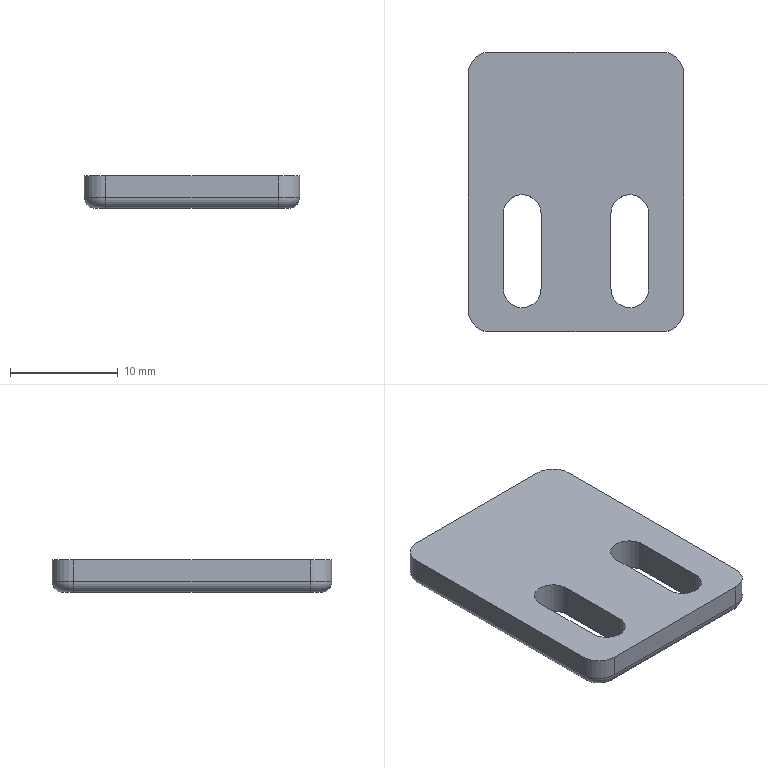Part | NX | 1 solid | 26 faces | box 20 x 26 x 3 mm | volume 1326 mm3 | cylinder 12 | plane 10 | torus 4 | commonest cylinder face diameters 2 x4 3.5 x4 4 x4
STEP:
#1=CARTESIAN_POINT('',(-3.25,-2.,1.5));
#2=VERTEX_POINT('',#1);
#3=CARTESIAN_POINT('',(-6.75,-2.,1.5));
#4=VERTEX_POINT('',#3);
#5=CARTESIAN_POINT('',(-5.,-2.,1.5));
#6=DIRECTION('',(0.,0.,1.));
#7=DIRECTION('',(1.,0.,0.));
#8=AXIS2_PLACEMENT_3D('',#5,#6,#7);
#9=CIRCLE('',#8,1.75);
#10=EDGE_CURVE('',#2,#4,#9,.T.);
#11=ORIENTED_EDGE('',*,*,#10,.F.);
#12=CARTESIAN_POINT('',(-3.25,-9.,1.5));
#13=VERTEX_POINT('',#12);
#14=CARTESIAN_POINT('',(-3.25,-2.,1.5));
#15=DIRECTION('',(0.,1.,0.));
#16=VECTOR('',#15,1000.);
#17=LINE('',#14,#16);
#18=EDGE_CURVE('',#13,#2,#17,.T.);
#19=ORIENTED_EDGE('',*,*,#18,.F.);
#20=CARTESIAN_POINT('',(-6.75,-9.,1.5));
#21=VERTEX_POINT('',#20);
#22=CARTESIAN_POINT('',(-5.,-9.,1.5));
#23=DIRECTION('',(0.,0.,1.));
#24=DIRECTION('',(1.,0.,0.));
#25=AXIS2_PLACEMENT_3D('',#22,#23,#24);
#26=CIRCLE('',#25,1.75);
#27=EDGE_CURVE('',#21,#13,#26,.T.);
#28=ORIENTED_EDGE('',*,*,#27,.F.);
#29=CARTESIAN_POINT('',(-6.75,-2.,1.5));
#30=DIRECTION('',(0.,-1.,0.));
#31=VECTOR('',#30,1000.);
#32=LINE('',#29,#31);
#33=EDGE_CURVE('',#4,#21,#32,.T.);
#34=ORIENTED_EDGE('',*,*,#33,.F.);
#35=EDGE_LOOP('',(#11,#19,#28,#34));
#36=FACE_BOUND('',#35,.T.);
#37=CARTESIAN_POINT('',(-10.,11.,1.5));
#38=VERTEX_POINT('',#37);
#39=CARTESIAN_POINT('',(-10.,-11.,1.5));
#40=VERTEX_POINT('',#39);
#41=CARTESIAN_POINT('',(-10.,13.,1.5));
#42=DIRECTION('',(0.,-1.,0.));
#43=VECTOR('',#42,1000.);
#44=LINE('',#41,#43);
#45=EDGE_CURVE('',#38,#40,#44,.T.);
#46=ORIENTED_EDGE('',*,*,#45,.T.);
#47=CARTESIAN_POINT('',(-8.,-13.,1.5));
#48=VERTEX_POINT('',#47);
#49=CARTESIAN_POINT('',(-8.,-11.,1.5));
#50=DIRECTION('',(0.,0.,-1.));
#51=DIRECTION('',(-1.,0.,0.));
#52=AXIS2_PLACEMENT_3D('',#49,#50,#51);
#53=CIRCLE('',#52,2.);
#54=EDGE_CURVE('',#40,#48,#53,.F.);
#55=ORIENTED_EDGE('',*,*,#54,.T.);
#56=CARTESIAN_POINT('',(8.,-13.,1.5));
#57=VERTEX_POINT('',#56);
#58=CARTESIAN_POINT('',(10.,-13.,1.5));
#59=DIRECTION('',(1.,0.,0.));
#60=VECTOR('',#59,1000.);
#61=LINE('',#58,#60);
#62=EDGE_CURVE('',#48,#57,#61,.T.);
#63=ORIENTED_EDGE('',*,*,#62,.T.);
#64=CARTESIAN_POINT('',(10.,-11.,1.5));
#65=VERTEX_POINT('',#64);
#66=CARTESIAN_POINT('',(8.,-11.,1.5));
#67=DIRECTION('',(0.,0.,-1.));
#68=DIRECTION('',(-1.,0.,0.));
#69=AXIS2_PLACEMENT_3D('',#66,#67,#68);
#70=CIRCLE('',#69,2.);
#71=EDGE_CURVE('',#57,#65,#70,.F.);
#72=ORIENTED_EDGE('',*,*,#71,.T.);
#73=CARTESIAN_POINT('',(10.,11.,1.5));
#74=VERTEX_POINT('',#73);
#75=CARTESIAN_POINT('',(10.,13.,1.5));
#76=DIRECTION('',(0.,1.,0.));
#77=VECTOR('',#76,1000.);
#78=LINE('',#75,#77);
#79=EDGE_CURVE('',#65,#74,#78,.T.);
#80=ORIENTED_EDGE('',*,*,#79,.T.);
#81=CARTESIAN_POINT('',(8.,13.,1.5));
#82=VERTEX_POINT('',#81);
#83=CARTESIAN_POINT('',(8.,11.,1.5));
#84=DIRECTION('',(0.,0.,-1.));
#85=DIRECTION('',(-1.,0.,0.));
#86=AXIS2_PLACEMENT_3D('',#83,#84,#85);
#87=CIRCLE('',#86,2.);
#88=EDGE_CURVE('',#74,#82,#87,.F.);
#89=ORIENTED_EDGE('',*,*,#88,.T.);
#90=CARTESIAN_POINT('',(-8.,13.,1.5));
#91=VERTEX_POINT('',#90);
#92=CARTESIAN_POINT('',(10.,13.,1.5));
#93=DIRECTION('',(-1.,0.,0.));
#94=VECTOR('',#93,1000.);
#95=LINE('',#92,#94);
#96=EDGE_CURVE('',#82,#91,#95,.T.);
#97=ORIENTED_EDGE('',*,*,#96,.T.);
#98=CARTESIAN_POINT('',(-8.,11.,1.5));
#99=DIRECTION('',(0.,0.,-1.));
#100=DIRECTION('',(-1.,0.,0.));
#101=AXIS2_PLACEMENT_3D('',#98,#99,#100);
#102=CIRCLE('',#101,2.);
#103=EDGE_CURVE('',#91,#38,#102,.F.);
#104=ORIENTED_EDGE('',*,*,#103,.T.);
#105=EDGE_LOOP('',(#46,#55,#63,#72,#80,#89,#97,#104));
#106=FACE_BOUND('',#105,.T.);
#107=CARTESIAN_POINT('',(6.75,-2.,1.5));
#108=VERTEX_POINT('',#107);
#109=CARTESIAN_POINT('',(3.25,-2.,1.5));
#110=VERTEX_POINT('',#109);
#111=CARTESIAN_POINT('',(5.,-2.,1.5));
#112=DIRECTION('',(0.,0.,1.));
#113=DIRECTION('',(-1.,0.,0.));
#114=AXIS2_PLACEMENT_3D('',#111,#112,#113);
#115=CIRCLE('',#114,1.75);
#116=EDGE_CURVE('',#108,#110,#115,.T.);
#117=ORIENTED_EDGE('',*,*,#116,.F.);
#118=CARTESIAN_POINT('',(6.75,-9.,1.5));
#119=VERTEX_POINT('',#118);
#120=CARTESIAN_POINT('',(6.75,-2.,1.5));
#121=DIRECTION('',(0.,1.,0.));
#122=VECTOR('',#121,1000.);
#123=LINE('',#120,#122);
#124=EDGE_CURVE('',#119,#108,#123,.T.);
#125=ORIENTED_EDGE('',*,*,#124,.F.);
#126=CARTESIAN_POINT('',(3.25,-9.,1.5));
#127=VERTEX_POINT('',#126);
#128=CARTESIAN_POINT('',(5.,-9.,1.5));
#129=DIRECTION('',(0.,0.,1.));
#130=DIRECTION('',(-1.,0.,0.));
#131=AXIS2_PLACEMENT_3D('',#128,#129,#130);
#132=CIRCLE('',#131,1.75);
#133=EDGE_CURVE('',#127,#119,#132,.T.);
#134=ORIENTED_EDGE('',*,*,#133,.F.);
#135=CARTESIAN_POINT('',(3.25,-2.,1.5));
#136=DIRECTION('',(0.,-1.,0.));
#137=VECTOR('',#136,1000.);
#138=LINE('',#135,#137);
#139=EDGE_CURVE('',#110,#127,#138,.T.);
#140=ORIENTED_EDGE('',*,*,#139,.F.);
#141=EDGE_LOOP('',(#117,#125,#134,#140));
#142=FACE_BOUND('',#141,.T.);
#143=CARTESIAN_POINT('',(0.,0.,1.5));
#144=DIRECTION('',(0.,0.,-1.));
#145=DIRECTION('',(-1.,0.,0.));
#146=AXIS2_PLACEMENT_3D('',#143,#144,#145);
#147=PLANE('',#146);
#148=ADVANCED_FACE('',(#36,#106,#142),#147,.F.);
#149=CARTESIAN_POINT('',(-8.,12.,-1.5));
#150=VERTEX_POINT('',#149);
#151=CARTESIAN_POINT('',(8.,12.,-1.5));
#152=VERTEX_POINT('',#151);
#153=CARTESIAN_POINT('',(8.,12.,-1.5));
#154=DIRECTION('',(-1.,0.,0.));
#155=VECTOR('',#154,1000.);
#156=LINE('',#153,#155);
#157=EDGE_CURVE('',#150,#152,#156,.F.);
#158=ORIENTED_EDGE('',*,*,#157,.T.);
#159=CARTESIAN_POINT('',(9.,11.,-1.5));
#160=VERTEX_POINT('',#159);
#161=CARTESIAN_POINT('',(8.,11.,-1.5));
#162=DIRECTION('',(0.,0.,-1.));
#163=DIRECTION('',(-1.,0.,0.));
#164=AXIS2_PLACEMENT_3D('',#161,#162,#163);
#165=CIRCLE('',#164,1.);
#166=EDGE_CURVE('',#152,#160,#165,.T.);
#167=ORIENTED_EDGE('',*,*,#166,.T.);
#168=CARTESIAN_POINT('',(9.,-11.,-1.5));
#169=VERTEX_POINT('',#168);
#170=CARTESIAN_POINT('',(9.,-11.,-1.5));
#171=DIRECTION('',(0.,1.,0.));
#172=VECTOR('',#171,1000.);
#173=LINE('',#170,#172);
#174=EDGE_CURVE('',#160,#169,#173,.F.);
#175=ORIENTED_EDGE('',*,*,#174,.T.);
#176=CARTESIAN_POINT('',(8.,-12.,-1.5));
#177=VERTEX_POINT('',#176);
#178=CARTESIAN_POINT('',(8.,-11.,-1.5));
#179=DIRECTION('',(0.,0.,-1.));
#180=DIRECTION('',(-1.,0.,0.));
#181=AXIS2_PLACEMENT_3D('',#178,#179,#180);
#182=CIRCLE('',#181,1.);
#183=EDGE_CURVE('',#169,#177,#182,.T.);
#184=ORIENTED_EDGE('',*,*,#183,.T.);
#185=CARTESIAN_POINT('',(-8.,-12.,-1.5));
#186=VERTEX_POINT('',#185);
#187=CARTESIAN_POINT('',(-8.,-12.,-1.5));
#188=DIRECTION('',(1.,0.,0.));
#189=VECTOR('',#188,1000.);
#190=LINE('',#187,#189);
#191=EDGE_CURVE('',#177,#186,#190,.F.);
#192=ORIENTED_EDGE('',*,*,#191,.T.);
#193=CARTESIAN_POINT('',(-9.,-11.,-1.5));
#194=VERTEX_POINT('',#193);
#195=CARTESIAN_POINT('',(-8.,-11.,-1.5));
#196=DIRECTION('',(0.,0.,-1.));
#197=DIRECTION('',(-1.,0.,0.));
#198=AXIS2_PLACEMENT_3D('',#195,#196,#197);
#199=CIRCLE('',#198,1.);
#200=EDGE_CURVE('',#186,#194,#199,.T.);
#201=ORIENTED_EDGE('',*,*,#200,.T.);
#202=CARTESIAN_POINT('',(-9.,11.,-1.5));
#203=VERTEX_POINT('',#202);
#204=CARTESIAN_POINT('',(-9.,11.,-1.5));
#205=DIRECTION('',(0.,-1.,0.));
#206=VECTOR('',#205,1000.);
#207=LINE('',#204,#206);
#208=EDGE_CURVE('',#194,#203,#207,.F.);
#209=ORIENTED_EDGE('',*,*,#208,.T.);
#210=CARTESIAN_POINT('',(-8.,11.,-1.5));
#211=DIRECTION('',(0.,0.,-1.));
#212=DIRECTION('',(-1.,0.,0.));
#213=AXIS2_PLACEMENT_3D('',#210,#211,#212);
#214=CIRCLE('',#213,1.);
#215=EDGE_CURVE('',#203,#150,#214,.T.);
#216=ORIENTED_EDGE('',*,*,#215,.T.);
#217=EDGE_LOOP('',(#158,#167,#175,#184,#192,#201,#209,#216));
#218=FACE_BOUND('',#217,.T.);
#219=CARTESIAN_POINT('',(-3.25,-9.,-1.5));
#220=VERTEX_POINT('',#219);
#221=CARTESIAN_POINT('',(-3.25,-2.,-1.5));
#222=VERTEX_POINT('',#221);
#223=CARTESIAN_POINT('',(-3.25,-2.,-1.5));
#224=DIRECTION('',(0.,1.,0.));
#225=VECTOR('',#224,1000.);
#226=LINE('',#223,#225);
#227=EDGE_CURVE('',#220,#222,#226,.T.);
#228=ORIENTED_EDGE('',*,*,#227,.T.);
#229=CARTESIAN_POINT('',(-6.75,-2.,-1.5));
#230=VERTEX_POINT('',#229);
#231=CARTESIAN_POINT('',(-5.,-2.,-1.5));
#232=DIRECTION('',(0.,0.,1.));
#233=DIRECTION('',(1.,0.,0.));
#234=AXIS2_PLACEMENT_3D('',#231,#232,#233);
#235=CIRCLE('',#234,1.75);
#236=EDGE_CURVE('',#222,#230,#235,.T.);
#237=ORIENTED_EDGE('',*,*,#236,.T.);
#238=CARTESIAN_POINT('',(-6.75,-9.,-1.5));
#239=VERTEX_POINT('',#238);
#240=CARTESIAN_POINT('',(-6.75,-2.,-1.5));
#241=DIRECTION('',(0.,-1.,0.));
#242=VECTOR('',#241,1000.);
#243=LINE('',#240,#242);
#244=EDGE_CURVE('',#230,#239,#243,.T.);
#245=ORIENTED_EDGE('',*,*,#244,.T.);
#246=CARTESIAN_POINT('',(-5.,-9.,-1.5));
#247=DIRECTION('',(0.,0.,1.));
#248=DIRECTION('',(1.,0.,0.));
#249=AXIS2_PLACEMENT_3D('',#246,#247,#248);
#250=CIRCLE('',#249,1.75);
#251=EDGE_CURVE('',#239,#220,#250,.T.);
#252=ORIENTED_EDGE('',*,*,#251,.T.);
#253=EDGE_LOOP('',(#228,#237,#245,#252));
#254=FACE_BOUND('',#253,.T.);
#255=CARTESIAN_POINT('',(6.75,-9.,-1.5));
#256=VERTEX_POINT('',#255);
#257=CARTESIAN_POINT('',(6.75,-2.,-1.5));
#258=VERTEX_POINT('',#257);
#259=CARTESIAN_POINT('',(6.75,-2.,-1.5));
#260=DIRECTION('',(0.,1.,0.));
#261=VECTOR('',#260,1000.);
#262=LINE('',#259,#261);
#263=EDGE_CURVE('',#256,#258,#262,.T.);
#264=ORIENTED_EDGE('',*,*,#263,.T.);
#265=CARTESIAN_POINT('',(3.25,-2.,-1.5));
#266=VERTEX_POINT('',#265);
#267=CARTESIAN_POINT('',(5.,-2.,-1.5));
#268=DIRECTION('',(0.,0.,1.));
#269=DIRECTION('',(-1.,0.,0.));
#270=AXIS2_PLACEMENT_3D('',#267,#268,#269);
#271=CIRCLE('',#270,1.75);
#272=EDGE_CURVE('',#258,#266,#271,.T.);
#273=ORIENTED_EDGE('',*,*,#272,.T.);
#274=CARTESIAN_POINT('',(3.25,-9.,-1.5));
#275=VERTEX_POINT('',#274);
#276=CARTESIAN_POINT('',(3.25,-2.,-1.5));
#277=DIRECTION('',(0.,-1.,0.));
#278=VECTOR('',#277,1000.);
#279=LINE('',#276,#278);
#280=EDGE_CURVE('',#266,#275,#279,.T.);
#281=ORIENTED_EDGE('',*,*,#280,.T.);
#282=CARTESIAN_POINT('',(5.,-9.,-1.5));
#283=DIRECTION('',(0.,0.,1.));
#284=DIRECTION('',(-1.,0.,0.));
#285=AXIS2_PLACEMENT_3D('',#282,#283,#284);
#286=CIRCLE('',#285,1.75);
#287=EDGE_CURVE('',#275,#256,#286,.T.);
#288=ORIENTED_EDGE('',*,*,#287,.T.);
#289=EDGE_LOOP('',(#264,#273,#281,#288));
#290=FACE_BOUND('',#289,.T.);
#291=CARTESIAN_POINT('',(0.,0.,-1.5));
#292=DIRECTION('',(0.,0.,-1.));
#293=DIRECTION('',(-1.,0.,0.));
#294=AXIS2_PLACEMENT_3D('',#291,#292,#293);
#295=PLANE('',#294);
#296=ADVANCED_FACE('',(#218,#254,#290),#295,.T.);
#297=CARTESIAN_POINT('',(-10.,11.,-0.5));
#298=VERTEX_POINT('',#297);
#299=CARTESIAN_POINT('',(-10.,11.,1.5));
#300=DIRECTION('',(0.,0.,-1.));
#301=VECTOR('',#300,1000.);
#302=LINE('',#299,#301);
#303=EDGE_CURVE('',#38,#298,#302,.T.);
#304=ORIENTED_EDGE('',*,*,#303,.T.);
#305=CARTESIAN_POINT('',(-10.,-11.,-0.5));
#306=VERTEX_POINT('',#305);
#307=CARTESIAN_POINT('',(-10.,-11.,-0.5));
#308=DIRECTION('',(0.,-1.,0.));
#309=VECTOR('',#308,1000.);
#310=LINE('',#307,#309);
#311=EDGE_CURVE('',#298,#306,#310,.T.);
#312=ORIENTED_EDGE('',*,*,#311,.T.);
#313=CARTESIAN_POINT('',(-10.,-11.,1.5));
#314=DIRECTION('',(0.,0.,-1.));
#315=VECTOR('',#314,1000.);
#316=LINE('',#313,#315);
#317=EDGE_CURVE('',#306,#40,#316,.F.);
#318=ORIENTED_EDGE('',*,*,#317,.T.);
#319=ORIENTED_EDGE('',*,*,#45,.F.);
#320=EDGE_LOOP('',(#304,#312,#318,#319));
#321=FACE_BOUND('',#320,.T.);
#322=CARTESIAN_POINT('',(-10.,13.,1.5));
#323=DIRECTION('',(1.,0.,0.));
#324=DIRECTION('',(0.,1.,0.));
#325=AXIS2_PLACEMENT_3D('',#322,#323,#324);
#326=PLANE('',#325);
#327=ADVANCED_FACE('',(#321),#326,.F.);
#328=CARTESIAN_POINT('',(-8.,-13.,-0.5));
#329=VERTEX_POINT('',#328);
#330=CARTESIAN_POINT('',(-8.,-13.,1.5));
#331=DIRECTION('',(0.,0.,-1.));
#332=VECTOR('',#331,1000.);
#333=LINE('',#330,#332);
#334=EDGE_CURVE('',#48,#329,#333,.T.);
#335=ORIENTED_EDGE('',*,*,#334,.T.);
#336=CARTESIAN_POINT('',(8.,-13.,-0.5));
#337=VERTEX_POINT('',#336);
#338=CARTESIAN_POINT('',(8.,-13.,-0.5));
#339=DIRECTION('',(1.,0.,0.));
#340=VECTOR('',#339,1000.);
#341=LINE('',#338,#340);
#342=EDGE_CURVE('',#329,#337,#341,.T.);
#343=ORIENTED_EDGE('',*,*,#342,.T.);
#344=CARTESIAN_POINT('',(8.,-13.,1.5));
#345=DIRECTION('',(0.,0.,-1.));
#346=VECTOR('',#345,1000.);
#347=LINE('',#344,#346);
#348=EDGE_CURVE('',#337,#57,#347,.F.);
#349=ORIENTED_EDGE('',*,*,#348,.T.);
#350=ORIENTED_EDGE('',*,*,#62,.F.);
#351=EDGE_LOOP('',(#335,#343,#349,#350));
#352=FACE_BOUND('',#351,.T.);
#353=CARTESIAN_POINT('',(10.,-13.,1.5));
#354=DIRECTION('',(0.,1.,0.));
#355=DIRECTION('',(-1.,0.,0.));
#356=AXIS2_PLACEMENT_3D('',#353,#354,#355);
#357=PLANE('',#356);
#358=ADVANCED_FACE('',(#352),#357,.F.);
#359=CARTESIAN_POINT('',(10.,-11.,-0.5));
#360=VERTEX_POINT('',#359);
#361=CARTESIAN_POINT('',(10.,-11.,1.5));
#362=DIRECTION('',(0.,0.,-1.));
#363=VECTOR('',#362,1000.);
#364=LINE('',#361,#363);
#365=EDGE_CURVE('',#65,#360,#364,.T.);
#366=ORIENTED_EDGE('',*,*,#365,.T.);
#367=CARTESIAN_POINT('',(10.,11.,-0.5));
#368=VERTEX_POINT('',#367);
#369=CARTESIAN_POINT('',(10.,11.,-0.5));
#370=DIRECTION('',(0.,1.,0.));
#371=VECTOR('',#370,1000.);
#372=LINE('',#369,#371);
#373=EDGE_CURVE('',#360,#368,#372,.T.);
#374=ORIENTED_EDGE('',*,*,#373,.T.);
#375=CARTESIAN_POINT('',(10.,11.,1.5));
#376=DIRECTION('',(0.,0.,-1.));
#377=VECTOR('',#376,1000.);
#378=LINE('',#375,#377);
#379=EDGE_CURVE('',#368,#74,#378,.F.);
#380=ORIENTED_EDGE('',*,*,#379,.T.);
#381=ORIENTED_EDGE('',*,*,#79,.F.);
#382=EDGE_LOOP('',(#366,#374,#380,#381));
#383=FACE_BOUND('',#382,.T.);
#384=CARTESIAN_POINT('',(10.,13.,1.5));
#385=DIRECTION('',(-1.,0.,0.));
#386=DIRECTION('',(0.,-1.,0.));
#387=AXIS2_PLACEMENT_3D('',#384,#385,#386);
#388=PLANE('',#387);
#389=ADVANCED_FACE('',(#383),#388,.F.);
#390=CARTESIAN_POINT('',(8.,13.,-0.5));
#391=VERTEX_POINT('',#390);
#392=CARTESIAN_POINT('',(8.,13.,1.5));
#393=DIRECTION('',(0.,0.,-1.));
#394=VECTOR('',#393,1000.);
#395=LINE('',#392,#394);
#396=EDGE_CURVE('',#82,#391,#395,.T.);
#397=ORIENTED_EDGE('',*,*,#396,.T.);
#398=CARTESIAN_POINT('',(-8.,13.,-0.5));
#399=VERTEX_POINT('',#398);
#400=CARTESIAN_POINT('',(-8.,13.,-0.5));
#401=DIRECTION('',(-1.,0.,0.));
#402=VECTOR('',#401,1000.);
#403=LINE('',#400,#402);
#404=EDGE_CURVE('',#391,#399,#403,.T.);
#405=ORIENTED_EDGE('',*,*,#404,.T.);
#406=CARTESIAN_POINT('',(-8.,13.,1.5));
#407=DIRECTION('',(0.,0.,-1.));
#408=VECTOR('',#407,1000.);
#409=LINE('',#406,#408);
#410=EDGE_CURVE('',#399,#91,#409,.F.);
#411=ORIENTED_EDGE('',*,*,#410,.T.);
#412=ORIENTED_EDGE('',*,*,#96,.F.);
#413=EDGE_LOOP('',(#397,#405,#411,#412));
#414=FACE_BOUND('',#413,.T.);
#415=CARTESIAN_POINT('',(10.,13.,1.5));
#416=DIRECTION('',(0.,-1.,0.));
#417=DIRECTION('',(1.,0.,0.));
#418=AXIS2_PLACEMENT_3D('',#415,#416,#417);
#419=PLANE('',#418);
#420=ADVANCED_FACE('',(#414),#419,.F.);
#421=ORIENTED_EDGE('',*,*,#236,.F.);
#422=CARTESIAN_POINT('',(-3.25,-2.,1.5));
#423=DIRECTION('',(0.,0.,-1.));
#424=VECTOR('',#423,1000.);
#425=LINE('',#422,#424);
#426=EDGE_CURVE('',#2,#222,#425,.T.);
#427=ORIENTED_EDGE('',*,*,#426,.F.);
#428=ORIENTED_EDGE('',*,*,#10,.T.);
#429=CARTESIAN_POINT('',(-6.75,-2.,1.5));
#430=DIRECTION('',(0.,0.,-1.));
#431=VECTOR('',#430,1000.);
#432=LINE('',#429,#431);
#433=EDGE_CURVE('',#4,#230,#432,.T.);
#434=ORIENTED_EDGE('',*,*,#433,.T.);
#435=EDGE_LOOP('',(#421,#427,#428,#434));
#436=FACE_BOUND('',#435,.T.);
#437=CARTESIAN_POINT('',(-5.,-2.,1.5));
#438=DIRECTION('',(0.,0.,-1.));
#439=DIRECTION('',(-1.,0.,0.));
#440=AXIS2_PLACEMENT_3D('',#437,#438,#439);
#441=CYLINDRICAL_SURFACE('',#440,1.75);
#442=ADVANCED_FACE('',(#436),#441,.F.);
#443=ORIENTED_EDGE('',*,*,#244,.F.);
#444=ORIENTED_EDGE('',*,*,#433,.F.);
#445=ORIENTED_EDGE('',*,*,#33,.T.);
#446=CARTESIAN_POINT('',(-6.75,-9.,1.5));
#447=DIRECTION('',(0.,0.,-1.));
#448=VECTOR('',#447,1000.);
#449=LINE('',#446,#448);
#450=EDGE_CURVE('',#21,#239,#449,.T.);
#451=ORIENTED_EDGE('',*,*,#450,.T.);
#452=EDGE_LOOP('',(#443,#444,#445,#451));
#453=FACE_BOUND('',#452,.T.);
#454=CARTESIAN_POINT('',(-6.75,-2.,1.5));
#455=DIRECTION('',(1.,0.,0.));
#456=DIRECTION('',(0.,0.,-1.));
#457=AXIS2_PLACEMENT_3D('',#454,#455,#456);
#458=PLANE('',#457);
#459=ADVANCED_FACE('',(#453),#458,.T.);
#460=ORIENTED_EDGE('',*,*,#251,.F.);
#461=ORIENTED_EDGE('',*,*,#450,.F.);
#462=ORIENTED_EDGE('',*,*,#27,.T.);
#463=CARTESIAN_POINT('',(-3.25,-9.,1.5));
#464=DIRECTION('',(0.,0.,-1.));
#465=VECTOR('',#464,1000.);
#466=LINE('',#463,#465);
#467=EDGE_CURVE('',#13,#220,#466,.T.);
#468=ORIENTED_EDGE('',*,*,#467,.T.);
#469=EDGE_LOOP('',(#460,#461,#462,#468));
#470=FACE_BOUND('',#469,.T.);
#471=CARTESIAN_POINT('',(-5.,-9.,1.5));
#472=DIRECTION('',(0.,0.,-1.));
#473=DIRECTION('',(-1.,0.,0.));
#474=AXIS2_PLACEMENT_3D('',#471,#472,#473);
#475=CYLINDRICAL_SURFACE('',#474,1.75);
#476=ADVANCED_FACE('',(#470),#475,.F.);
#477=ORIENTED_EDGE('',*,*,#227,.F.);
#478=ORIENTED_EDGE('',*,*,#467,.F.);
#479=ORIENTED_EDGE('',*,*,#18,.T.);
#480=ORIENTED_EDGE('',*,*,#426,.T.);
#481=EDGE_LOOP('',(#477,#478,#479,#480));
#482=FACE_BOUND('',#481,.T.);
#483=CARTESIAN_POINT('',(-3.25,-2.,1.5));
#484=DIRECTION('',(-1.,0.,0.));
#485=DIRECTION('',(0.,0.,1.));
#486=AXIS2_PLACEMENT_3D('',#483,#484,#485);
#487=PLANE('',#486);
#488=ADVANCED_FACE('',(#482),#487,.T.);
#489=ORIENTED_EDGE('',*,*,#272,.F.);
#490=CARTESIAN_POINT('',(6.75,-2.,1.5));
#491=DIRECTION('',(0.,0.,-1.));
#492=VECTOR('',#491,1000.);
#493=LINE('',#490,#492);
#494=EDGE_CURVE('',#108,#258,#493,.T.);
#495=ORIENTED_EDGE('',*,*,#494,.F.);
#496=ORIENTED_EDGE('',*,*,#116,.T.);
#497=CARTESIAN_POINT('',(3.25,-2.,1.5));
#498=DIRECTION('',(0.,0.,-1.));
#499=VECTOR('',#498,1000.);
#500=LINE('',#497,#499);
#501=EDGE_CURVE('',#110,#266,#500,.T.);
#502=ORIENTED_EDGE('',*,*,#501,.T.);
#503=EDGE_LOOP('',(#489,#495,#496,#502));
#504=FACE_BOUND('',#503,.T.);
#505=CARTESIAN_POINT('',(5.,-2.,1.5));
#506=DIRECTION('',(0.,0.,-1.));
#507=DIRECTION('',(-1.,0.,0.));
#508=AXIS2_PLACEMENT_3D('',#505,#506,#507);
#509=CYLINDRICAL_SURFACE('',#508,1.75);
#510=ADVANCED_FACE('',(#504),#509,.F.);
#511=ORIENTED_EDGE('',*,*,#280,.F.);
#512=ORIENTED_EDGE('',*,*,#501,.F.);
#513=ORIENTED_EDGE('',*,*,#139,.T.);
#514=CARTESIAN_POINT('',(3.25,-9.,1.5));
#515=DIRECTION('',(0.,0.,-1.));
#516=VECTOR('',#515,1000.);
#517=LINE('',#514,#516);
#518=EDGE_CURVE('',#127,#275,#517,.T.);
#519=ORIENTED_EDGE('',*,*,#518,.T.);
#520=EDGE_LOOP('',(#511,#512,#513,#519));
#521=FACE_BOUND('',#520,.T.);
#522=CARTESIAN_POINT('',(3.25,-2.,1.5));
#523=DIRECTION('',(1.,0.,0.));
#524=DIRECTION('',(0.,0.,-1.));
#525=AXIS2_PLACEMENT_3D('',#522,#523,#524);
#526=PLANE('',#525);
#527=ADVANCED_FACE('',(#521),#526,.T.);
#528=ORIENTED_EDGE('',*,*,#287,.F.);
#529=ORIENTED_EDGE('',*,*,#518,.F.);
#530=ORIENTED_EDGE('',*,*,#133,.T.);
#531=CARTESIAN_POINT('',(6.75,-9.,1.5));
#532=DIRECTION('',(0.,0.,-1.));
#533=VECTOR('',#532,1000.);
#534=LINE('',#531,#533);
#535=EDGE_CURVE('',#119,#256,#534,.T.);
#536=ORIENTED_EDGE('',*,*,#535,.T.);
#537=EDGE_LOOP('',(#528,#529,#530,#536));
#538=FACE_BOUND('',#537,.T.);
#539=CARTESIAN_POINT('',(5.,-9.,1.5));
#540=DIRECTION('',(0.,0.,-1.));
#541=DIRECTION('',(-1.,0.,0.));
#542=AXIS2_PLACEMENT_3D('',#539,#540,#541);
#543=CYLINDRICAL_SURFACE('',#542,1.75);
#544=ADVANCED_FACE('',(#538),#543,.F.);
#545=ORIENTED_EDGE('',*,*,#263,.F.);
#546=ORIENTED_EDGE('',*,*,#535,.F.);
#547=ORIENTED_EDGE('',*,*,#124,.T.);
#548=ORIENTED_EDGE('',*,*,#494,.T.);
#549=EDGE_LOOP('',(#545,#546,#547,#548));
#550=FACE_BOUND('',#549,.T.);
#551=CARTESIAN_POINT('',(6.75,-2.,1.5));
#552=DIRECTION('',(-1.,0.,0.));
#553=DIRECTION('',(0.,0.,1.));
#554=AXIS2_PLACEMENT_3D('',#551,#552,#553);
#555=PLANE('',#554);
#556=ADVANCED_FACE('',(#550),#555,.T.);
#557=ORIENTED_EDGE('',*,*,#317,.F.);
#558=CARTESIAN_POINT('',(-8.,-11.,-0.5));
#559=DIRECTION('',(0.,0.,-1.));
#560=DIRECTION('',(-1.,0.,0.));
#561=AXIS2_PLACEMENT_3D('',#558,#559,#560);
#562=CIRCLE('',#561,2.);
#563=EDGE_CURVE('',#306,#329,#562,.F.);
#564=ORIENTED_EDGE('',*,*,#563,.T.);
#565=ORIENTED_EDGE('',*,*,#334,.F.);
#566=ORIENTED_EDGE('',*,*,#54,.F.);
#567=EDGE_LOOP('',(#557,#564,#565,#566));
#568=FACE_BOUND('',#567,.T.);
#569=CARTESIAN_POINT('',(-8.,-11.,1.5));
#570=DIRECTION('',(0.,0.,-1.));
#571=DIRECTION('',(-1.,0.,0.));
#572=AXIS2_PLACEMENT_3D('',#569,#570,#571);
#573=CYLINDRICAL_SURFACE('',#572,2.);
#574=ADVANCED_FACE('',(#568),#573,.T.);
#575=ORIENTED_EDGE('',*,*,#348,.F.);
#576=CARTESIAN_POINT('',(8.,-11.,-0.5));
#577=DIRECTION('',(0.,0.,-1.));
#578=DIRECTION('',(-1.,0.,0.));
#579=AXIS2_PLACEMENT_3D('',#576,#577,#578);
#580=CIRCLE('',#579,2.);
#581=EDGE_CURVE('',#337,#360,#580,.F.);
#582=ORIENTED_EDGE('',*,*,#581,.T.);
#583=ORIENTED_EDGE('',*,*,#365,.F.);
#584=ORIENTED_EDGE('',*,*,#71,.F.);
#585=EDGE_LOOP('',(#575,#582,#583,#584));
#586=FACE_BOUND('',#585,.T.);
#587=CARTESIAN_POINT('',(8.,-11.,1.5));
#588=DIRECTION('',(0.,0.,-1.));
#589=DIRECTION('',(-1.,0.,0.));
#590=AXIS2_PLACEMENT_3D('',#587,#588,#589);
#591=CYLINDRICAL_SURFACE('',#590,2.);
#592=ADVANCED_FACE('',(#586),#591,.T.);
#593=ORIENTED_EDGE('',*,*,#410,.F.);
#594=CARTESIAN_POINT('',(-8.,11.,-0.5));
#595=DIRECTION('',(0.,0.,-1.));
#596=DIRECTION('',(-1.,0.,0.));
#597=AXIS2_PLACEMENT_3D('',#594,#595,#596);
#598=CIRCLE('',#597,2.);
#599=EDGE_CURVE('',#399,#298,#598,.F.);
#600=ORIENTED_EDGE('',*,*,#599,.T.);
#601=ORIENTED_EDGE('',*,*,#303,.F.);
#602=ORIENTED_EDGE('',*,*,#103,.F.);
#603=EDGE_LOOP('',(#593,#600,#601,#602));
#604=FACE_BOUND('',#603,.T.);
#605=CARTESIAN_POINT('',(-8.,11.,1.5));
#606=DIRECTION('',(0.,0.,-1.));
#607=DIRECTION('',(-1.,0.,0.));
#608=AXIS2_PLACEMENT_3D('',#605,#606,#607);
#609=CYLINDRICAL_SURFACE('',#608,2.);
#610=ADVANCED_FACE('',(#604),#609,.T.);
#611=ORIENTED_EDGE('',*,*,#379,.F.);
#612=CARTESIAN_POINT('',(8.,11.,-0.5));
#613=DIRECTION('',(0.,0.,-1.));
#614=DIRECTION('',(-1.,0.,0.));
#615=AXIS2_PLACEMENT_3D('',#612,#613,#614);
#616=CIRCLE('',#615,2.);
#617=EDGE_CURVE('',#368,#391,#616,.F.);
#618=ORIENTED_EDGE('',*,*,#617,.T.);
#619=ORIENTED_EDGE('',*,*,#396,.F.);
#620=ORIENTED_EDGE('',*,*,#88,.F.);
#621=EDGE_LOOP('',(#611,#618,#619,#620));
#622=FACE_BOUND('',#621,.T.);
#623=CARTESIAN_POINT('',(8.,11.,1.5));
#624=DIRECTION('',(0.,0.,-1.));
#625=DIRECTION('',(-1.,0.,0.));
#626=AXIS2_PLACEMENT_3D('',#623,#624,#625);
#627=CYLINDRICAL_SURFACE('',#626,2.);
#628=ADVANCED_FACE('',(#622),#627,.T.);
#629=CARTESIAN_POINT('',(-8.,-12.,-0.5));
#630=DIRECTION('',(1.,0.,0.));
#631=DIRECTION('',(0.,0.,-1.));
#632=AXIS2_PLACEMENT_3D('',#629,#630,#631);
#633=CIRCLE('',#632,1.);
#634=EDGE_CURVE('',#329,#186,#633,.T.);
#635=ORIENTED_EDGE('',*,*,#634,.F.);
#636=ORIENTED_EDGE('',*,*,#563,.F.);
#637=CARTESIAN_POINT('',(-9.,-11.,-0.5));
#638=DIRECTION('',(0.,1.,0.));
#639=DIRECTION('',(-1.,0.,0.));
#640=AXIS2_PLACEMENT_3D('',#637,#638,#639);
#641=CIRCLE('',#640,1.);
#642=EDGE_CURVE('',#194,#306,#641,.T.);
#643=ORIENTED_EDGE('',*,*,#642,.F.);
#644=ORIENTED_EDGE('',*,*,#200,.F.);
#645=EDGE_LOOP('',(#635,#636,#643,#644));
#646=FACE_BOUND('',#645,.T.);
#647=CARTESIAN_POINT('',(-8.,-11.,-0.5));
#648=DIRECTION('',(0.,0.,-1.));
#649=DIRECTION('',(-1.,0.,0.));
#650=AXIS2_PLACEMENT_3D('',#647,#648,#649);
#651=TOROIDAL_SURFACE('',#650,1.,1.);
#652=ADVANCED_FACE('',(#646),#651,.T.);
#653=ORIENTED_EDGE('',*,*,#642,.T.);
#654=ORIENTED_EDGE('',*,*,#311,.F.);
#655=CARTESIAN_POINT('',(-9.,11.,-0.5));
#656=DIRECTION('',(0.,1.,0.));
#657=DIRECTION('',(0.,0.,1.));
#658=AXIS2_PLACEMENT_3D('',#655,#656,#657);
#659=CIRCLE('',#658,1.);
#660=EDGE_CURVE('',#203,#298,#659,.T.);
#661=ORIENTED_EDGE('',*,*,#660,.F.);
#662=ORIENTED_EDGE('',*,*,#208,.F.);
#663=EDGE_LOOP('',(#653,#654,#661,#662));
#664=FACE_BOUND('',#663,.T.);
#665=CARTESIAN_POINT('',(-9.,13.,-0.5));
#666=DIRECTION('',(0.,1.,0.));
#667=DIRECTION('',(-1.,0.,0.));
#668=AXIS2_PLACEMENT_3D('',#665,#666,#667);
#669=CYLINDRICAL_SURFACE('',#668,1.);
#670=ADVANCED_FACE('',(#664),#669,.T.);
#671=ORIENTED_EDGE('',*,*,#634,.T.);
#672=ORIENTED_EDGE('',*,*,#191,.F.);
#673=CARTESIAN_POINT('',(8.,-12.,-0.5));
#674=DIRECTION('',(1.,0.,0.));
#675=DIRECTION('',(0.,0.,-1.));
#676=AXIS2_PLACEMENT_3D('',#673,#674,#675);
#677=CIRCLE('',#676,1.);
#678=EDGE_CURVE('',#337,#177,#677,.T.);
#679=ORIENTED_EDGE('',*,*,#678,.F.);
#680=ORIENTED_EDGE('',*,*,#342,.F.);
#681=EDGE_LOOP('',(#671,#672,#679,#680));
#682=FACE_BOUND('',#681,.T.);
#683=CARTESIAN_POINT('',(10.,-12.,-0.5));
#684=DIRECTION('',(-1.,0.,0.));
#685=DIRECTION('',(0.,-1.,0.));
#686=AXIS2_PLACEMENT_3D('',#683,#684,#685);
#687=CYLINDRICAL_SURFACE('',#686,1.);
#688=ADVANCED_FACE('',(#682),#687,.T.);
#689=ORIENTED_EDGE('',*,*,#660,.T.);
#690=ORIENTED_EDGE('',*,*,#599,.F.);
#691=CARTESIAN_POINT('',(-8.,12.,-0.5));
#692=DIRECTION('',(1.,0.,0.));
#693=DIRECTION('',(0.,1.,0.));
#694=AXIS2_PLACEMENT_3D('',#691,#692,#693);
#695=CIRCLE('',#694,1.);
#696=EDGE_CURVE('',#150,#399,#695,.T.);
#697=ORIENTED_EDGE('',*,*,#696,.F.);
#698=ORIENTED_EDGE('',*,*,#215,.F.);
#699=EDGE_LOOP('',(#689,#690,#697,#698));
#700=FACE_BOUND('',#699,.T.);
#701=CARTESIAN_POINT('',(-8.,11.,-0.5));
#702=DIRECTION('',(0.,0.,-1.));
#703=DIRECTION('',(-1.,0.,0.));
#704=AXIS2_PLACEMENT_3D('',#701,#702,#703);
#705=TOROIDAL_SURFACE('',#704,1.,1.);
#706=ADVANCED_FACE('',(#700),#705,.T.);
#707=ORIENTED_EDGE('',*,*,#678,.T.);
#708=ORIENTED_EDGE('',*,*,#183,.F.);
#709=CARTESIAN_POINT('',(9.,-11.,-0.5));
#710=DIRECTION('',(0.,1.,0.));
#711=DIRECTION('',(0.,0.,1.));
#712=AXIS2_PLACEMENT_3D('',#709,#710,#711);
#713=CIRCLE('',#712,1.);
#714=EDGE_CURVE('',#360,#169,#713,.T.);
#715=ORIENTED_EDGE('',*,*,#714,.F.);
#716=ORIENTED_EDGE('',*,*,#581,.F.);
#717=EDGE_LOOP('',(#707,#708,#715,#716));
#718=FACE_BOUND('',#717,.T.);
#719=CARTESIAN_POINT('',(8.,-11.,-0.5));
#720=DIRECTION('',(0.,0.,-1.));
#721=DIRECTION('',(-1.,0.,0.));
#722=AXIS2_PLACEMENT_3D('',#719,#720,#721);
#723=TOROIDAL_SURFACE('',#722,1.,1.);
#724=ADVANCED_FACE('',(#718),#723,.T.);
#725=ORIENTED_EDGE('',*,*,#696,.T.);
#726=ORIENTED_EDGE('',*,*,#404,.F.);
#727=CARTESIAN_POINT('',(8.,12.,-0.5));
#728=DIRECTION('',(1.,0.,0.));
#729=DIRECTION('',(0.,0.,-1.));
#730=AXIS2_PLACEMENT_3D('',#727,#728,#729);
#731=CIRCLE('',#730,1.);
#732=EDGE_CURVE('',#152,#391,#731,.T.);
#733=ORIENTED_EDGE('',*,*,#732,.F.);
#734=ORIENTED_EDGE('',*,*,#157,.F.);
#735=EDGE_LOOP('',(#725,#726,#733,#734));
#736=FACE_BOUND('',#735,.T.);
#737=CARTESIAN_POINT('',(10.,12.,-0.5));
#738=DIRECTION('',(1.,0.,0.));
#739=DIRECTION('',(0.,1.,0.));
#740=AXIS2_PLACEMENT_3D('',#737,#738,#739);
#741=CYLINDRICAL_SURFACE('',#740,1.);
#742=ADVANCED_FACE('',(#736),#741,.T.);
#743=ORIENTED_EDGE('',*,*,#714,.T.);
#744=ORIENTED_EDGE('',*,*,#174,.F.);
#745=CARTESIAN_POINT('',(9.,11.,-0.5));
#746=DIRECTION('',(0.,1.,0.));
#747=DIRECTION('',(0.,0.,1.));
#748=AXIS2_PLACEMENT_3D('',#745,#746,#747);
#749=CIRCLE('',#748,1.);
#750=EDGE_CURVE('',#368,#160,#749,.T.);
#751=ORIENTED_EDGE('',*,*,#750,.F.);
#752=ORIENTED_EDGE('',*,*,#373,.F.);
#753=EDGE_LOOP('',(#743,#744,#751,#752));
#754=FACE_BOUND('',#753,.T.);
#755=CARTESIAN_POINT('',(9.,13.,-0.5));
#756=DIRECTION('',(0.,-1.,0.));
#757=DIRECTION('',(1.,0.,0.));
#758=AXIS2_PLACEMENT_3D('',#755,#756,#757);
#759=CYLINDRICAL_SURFACE('',#758,1.);
#760=ADVANCED_FACE('',(#754),#759,.T.);
#761=ORIENTED_EDGE('',*,*,#732,.T.);
#762=ORIENTED_EDGE('',*,*,#617,.F.);
#763=ORIENTED_EDGE('',*,*,#750,.T.);
#764=ORIENTED_EDGE('',*,*,#166,.F.);
#765=EDGE_LOOP('',(#761,#762,#763,#764));
#766=FACE_BOUND('',#765,.T.);
#767=CARTESIAN_POINT('',(8.,11.,-0.5));
#768=DIRECTION('',(0.,0.,-1.));
#769=DIRECTION('',(-1.,0.,0.));
#770=AXIS2_PLACEMENT_3D('',#767,#768,#769);
#771=TOROIDAL_SURFACE('',#770,1.,1.);
#772=ADVANCED_FACE('',(#766),#771,.T.);
#773=CLOSED_SHELL('',(#148,#296,#327,#358,#389,#420,#442,#459,#476,#488,#510,#527,#544,#556,#574,#592,#610,#628,#652,#670,#688,#706,#724,#742,#760,#772));
#774=MANIFOLD_SOLID_BREP('',#773);
#775=(LENGTH_UNIT()NAMED_UNIT(*)SI_UNIT(.MILLI.,.METRE.));
#776=UNCERTAINTY_MEASURE_WITH_UNIT(LENGTH_MEASURE(0.00001),#775,'','');
#777=(NAMED_UNIT(*)PLANE_ANGLE_UNIT()SI_UNIT($,.RADIAN.));
#778=(NAMED_UNIT(*)SI_UNIT($,.STERADIAN.)SOLID_ANGLE_UNIT());
#779=(GEOMETRIC_REPRESENTATION_CONTEXT(3)GLOBAL_UNCERTAINTY_ASSIGNED_CONTEXT((#776))GLOBAL_UNIT_ASSIGNED_CONTEXT((#775,#777,#778))REPRESENTATION_CONTEXT('',''));
#780=ADVANCED_BREP_SHAPE_REPRESENTATION('',(#774),#779);